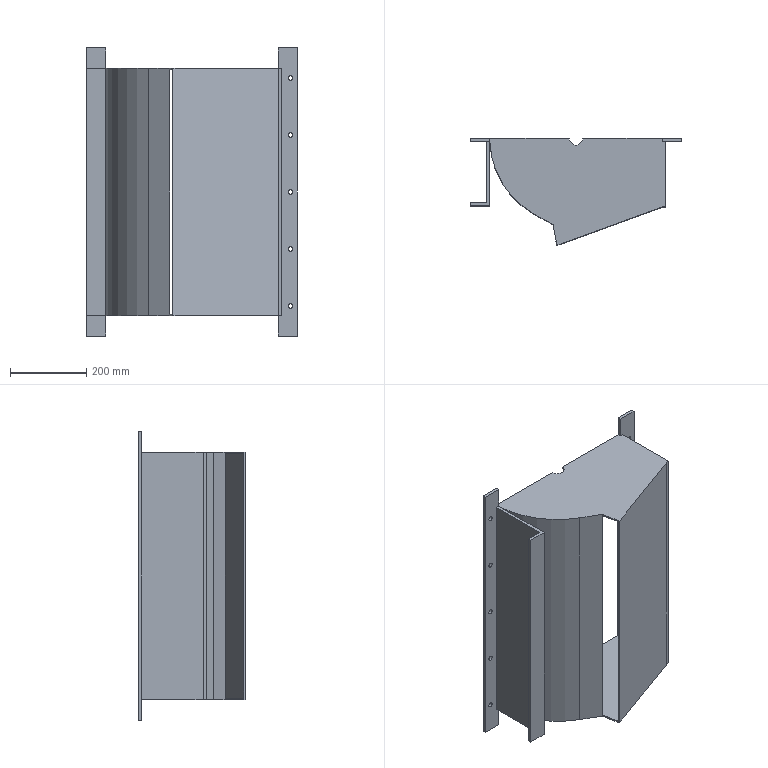Part | SolidWorks | features ICE 8, LPattern 2, Extrusion 1 | 1 solid | 58 faces | box 554 x 280.82 x 758 mm | volume 5312644 mm3 | plane 34 | cylinder 24 | commonest cylinder face diameters 12 x20 35 x2 446 x1 454 x1